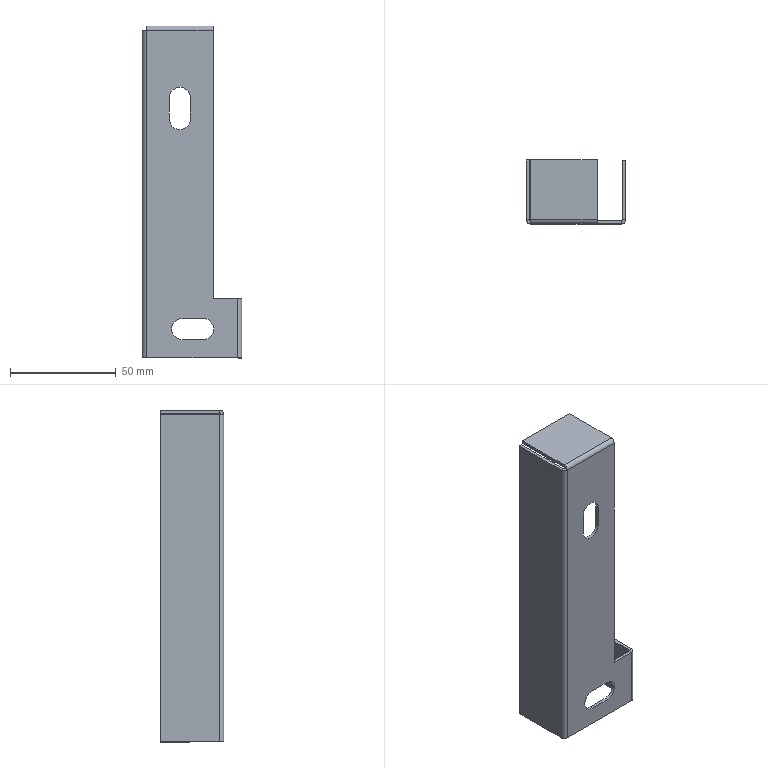Part | SolidWorks | features ICE 4, EdgeFlange 3, Cut 1, FlatPattern 1, SMBaseFlange 1, SheetMetal 1 | 1 solid | 41 faces | box 47 x 30 x 157 mm | volume 16912 mm3 | plane 30 | cylinder 11 | commonest cylinder face diameters 10 x5 1 x3 4 x3
STEP:
#1=CARTESIAN_POINT('',(17.75,0.,128.));
#2=VERTEX_POINT('',#1);
#3=CARTESIAN_POINT('',(22.75,0.,123.));
#4=VERTEX_POINT('',#3);
#5=CARTESIAN_POINT('',(17.75,0.,123.));
#6=DIRECTION('',(0.,1.,0.));
#7=DIRECTION('',(0.,0.,1.));
#8=AXIS2_PLACEMENT_3D('',#5,#6,#7);
#9=CIRCLE('',#8,5.);
#10=EDGE_CURVE('',#2,#4,#9,.T.);
#11=ORIENTED_EDGE('',*,*,#10,.F.);
#12=CARTESIAN_POINT('',(17.75,1.5,128.));
#13=VERTEX_POINT('',#12);
#14=CARTESIAN_POINT('',(17.75,-8.5,128.));
#15=DIRECTION('',(0.,1.,0.));
#16=VECTOR('',#15,1000.);
#17=LINE('',#14,#16);
#18=EDGE_CURVE('',#2,#13,#17,.T.);
#19=ORIENTED_EDGE('',*,*,#18,.T.);
#20=CARTESIAN_POINT('',(22.75,1.5,123.));
#21=VERTEX_POINT('',#20);
#22=CARTESIAN_POINT('',(17.75,1.5,123.));
#23=DIRECTION('',(0.,1.,0.));
#24=DIRECTION('',(0.,0.,1.));
#25=AXIS2_PLACEMENT_3D('',#22,#23,#24);
#26=CIRCLE('',#25,5.);
#27=EDGE_CURVE('',#13,#21,#26,.T.);
#28=ORIENTED_EDGE('',*,*,#27,.T.);
#29=CARTESIAN_POINT('',(22.75,-8.5,123.));
#30=DIRECTION('',(0.,1.,0.));
#31=VECTOR('',#30,1000.);
#32=LINE('',#29,#31);
#33=EDGE_CURVE('',#4,#21,#32,.T.);
#34=ORIENTED_EDGE('',*,*,#33,.F.);
#35=EDGE_LOOP('',(#11,#19,#28,#34));
#36=FACE_OUTER_BOUND('',#35,.T.);
#37=CARTESIAN_POINT('',(17.75,-8.5,123.));
#38=DIRECTION('',(0.,1.,0.));
#39=DIRECTION('',(0.,0.,1.));
#40=AXIS2_PLACEMENT_3D('',#37,#38,#39);
#41=CYLINDRICAL_SURFACE('',#40,5.);
#42=ADVANCED_FACE('',(#36),#41,.F.);
#43=CARTESIAN_POINT('',(33.5,1.5,28.));
#44=VERTEX_POINT('',#43);
#45=CARTESIAN_POINT('',(33.5,1.5,155.));
#46=VERTEX_POINT('',#45);
#47=CARTESIAN_POINT('',(33.5,1.5,155.));
#48=DIRECTION('',(0.,0.,1.));
#49=VECTOR('',#48,1000.);
#50=LINE('',#47,#49);
#51=EDGE_CURVE('',#44,#46,#50,.T.);
#52=ORIENTED_EDGE('',*,*,#51,.T.);
#53=CARTESIAN_POINT('',(33.5,0.,155.));
#54=VERTEX_POINT('',#53);
#55=CARTESIAN_POINT('',(33.5,1.5,155.));
#56=DIRECTION('',(0.,-1.,0.));
#57=VECTOR('',#56,1000.);
#58=LINE('',#55,#57);
#59=EDGE_CURVE('',#46,#54,#58,.T.);
#60=ORIENTED_EDGE('',*,*,#59,.T.);
#61=CARTESIAN_POINT('',(33.5,0.,28.));
#62=VERTEX_POINT('',#61);
#63=CARTESIAN_POINT('',(33.5,0.,157.));
#64=DIRECTION('',(0.,0.,1.));
#65=VECTOR('',#64,1000.);
#66=LINE('',#63,#65);
#67=EDGE_CURVE('',#62,#54,#66,.T.);
#68=ORIENTED_EDGE('',*,*,#67,.F.);
#69=CARTESIAN_POINT('',(33.5,0.,28.));
#70=DIRECTION('',(0.,1.,0.));
#71=VECTOR('',#70,1000.);
#72=LINE('',#69,#71);
#73=EDGE_CURVE('',#62,#44,#72,.T.);
#74=ORIENTED_EDGE('',*,*,#73,.T.);
#75=EDGE_LOOP('',(#52,#60,#68,#74));
#76=FACE_OUTER_BOUND('',#75,.T.);
#77=CARTESIAN_POINT('',(33.5,0.,157.));
#78=DIRECTION('',(-1.,0.,0.));
#79=DIRECTION('',(0.,0.,1.));
#80=AXIS2_PLACEMENT_3D('',#77,#78,#79);
#81=PLANE('',#80);
#82=ADVANCED_FACE('',(#76),#81,.F.);
#83=CARTESIAN_POINT('',(33.5,2.,157.));
#84=VERTEX_POINT('',#83);
#85=CARTESIAN_POINT('',(33.5,30.,157.));
#86=VERTEX_POINT('',#85);
#87=CARTESIAN_POINT('',(33.5,0.,157.));
#88=DIRECTION('',(0.,1.,0.));
#89=VECTOR('',#88,1000.);
#90=LINE('',#87,#89);
#91=EDGE_CURVE('',#84,#86,#90,.T.);
#92=ORIENTED_EDGE('',*,*,#91,.F.);
#93=CARTESIAN_POINT('',(33.5,2.,155.5));
#94=VERTEX_POINT('',#93);
#95=CARTESIAN_POINT('',(33.5,2.,157.));
#96=DIRECTION('',(0.,0.,-1.));
#97=VECTOR('',#96,1000.);
#98=LINE('',#95,#97);
#99=EDGE_CURVE('',#84,#94,#98,.T.);
#100=ORIENTED_EDGE('',*,*,#99,.T.);
#101=CARTESIAN_POINT('',(33.5,30.,155.5));
#102=VERTEX_POINT('',#101);
#103=CARTESIAN_POINT('',(33.5,0.,155.5));
#104=DIRECTION('',(0.,1.,0.));
#105=VECTOR('',#104,1000.);
#106=LINE('',#103,#105);
#107=EDGE_CURVE('',#94,#102,#106,.T.);
#108=ORIENTED_EDGE('',*,*,#107,.T.);
#109=CARTESIAN_POINT('',(33.5,30.,157.));
#110=DIRECTION('',(0.,0.,-1.));
#111=VECTOR('',#110,1000.);
#112=LINE('',#109,#111);
#113=EDGE_CURVE('',#86,#102,#112,.T.);
#114=ORIENTED_EDGE('',*,*,#113,.F.);
#115=EDGE_LOOP('',(#92,#100,#108,#114));
#116=FACE_OUTER_BOUND('',#115,.T.);
#117=CARTESIAN_POINT('',(33.5,0.,157.));
#118=DIRECTION('',(-1.,0.,0.));
#119=DIRECTION('',(0.,0.,1.));
#120=AXIS2_PLACEMENT_3D('',#117,#118,#119);
#121=PLANE('',#120);
#122=ADVANCED_FACE('',(#116),#121,.F.);
#123=CARTESIAN_POINT('',(0.,2.,155.));
#124=VERTEX_POINT('',#123);
#125=CARTESIAN_POINT('',(1.5,2.,155.));
#126=VERTEX_POINT('',#125);
#127=CARTESIAN_POINT('',(0.,2.,155.));
#128=DIRECTION('',(1.,0.,0.));
#129=VECTOR('',#128,1000.);
#130=LINE('',#127,#129);
#131=EDGE_CURVE('',#124,#126,#130,.T.);
#132=ORIENTED_EDGE('',*,*,#131,.F.);
#133=CARTESIAN_POINT('',(2.,0.,155.));
#134=VERTEX_POINT('',#133);
#135=CARTESIAN_POINT('',(2.,2.,155.));
#136=DIRECTION('',(0.,0.,1.));
#137=DIRECTION('',(-1.,0.,0.));
#138=AXIS2_PLACEMENT_3D('',#135,#136,#137);
#139=CIRCLE('',#138,2.);
#140=EDGE_CURVE('',#124,#134,#139,.T.);
#141=ORIENTED_EDGE('',*,*,#140,.T.);
#142=CARTESIAN_POINT('',(2.,1.5,155.));
#143=VERTEX_POINT('',#142);
#144=CARTESIAN_POINT('',(2.,1.5,155.));
#145=DIRECTION('',(0.,-1.,0.));
#146=VECTOR('',#145,1000.);
#147=LINE('',#144,#146);
#148=EDGE_CURVE('',#143,#134,#147,.T.);
#149=ORIENTED_EDGE('',*,*,#148,.F.);
#150=CARTESIAN_POINT('',(2.,2.,155.));
#151=DIRECTION('',(0.,0.,1.));
#152=DIRECTION('',(1.,0.,0.));
#153=AXIS2_PLACEMENT_3D('',#150,#151,#152);
#154=CIRCLE('',#153,0.5);
#155=EDGE_CURVE('',#126,#143,#154,.T.);
#156=ORIENTED_EDGE('',*,*,#155,.F.);
#157=EDGE_LOOP('',(#132,#141,#149,#156));
#158=FACE_OUTER_BOUND('',#157,.T.);
#159=CARTESIAN_POINT('',(0.,2.,155.));
#160=DIRECTION('',(0.,0.,1.));
#161=DIRECTION('',(1.,0.,0.));
#162=AXIS2_PLACEMENT_3D('',#159,#160,#161);
#163=PLANE('',#162);
#164=ADVANCED_FACE('',(#158),#163,.T.);
#165=CARTESIAN_POINT('',(0.,30.,155.));
#166=VERTEX_POINT('',#165);
#167=CARTESIAN_POINT('',(0.,30.,155.));
#168=DIRECTION('',(0.,-1.,0.));
#169=VECTOR('',#168,1000.);
#170=LINE('',#167,#169);
#171=EDGE_CURVE('',#166,#124,#170,.T.);
#172=ORIENTED_EDGE('',*,*,#171,.T.);
#173=ORIENTED_EDGE('',*,*,#131,.T.);
#174=CARTESIAN_POINT('',(1.5,30.,155.));
#175=VERTEX_POINT('',#174);
#176=CARTESIAN_POINT('',(1.5,30.,155.));
#177=DIRECTION('',(0.,-1.,0.));
#178=VECTOR('',#177,1000.);
#179=LINE('',#176,#178);
#180=EDGE_CURVE('',#175,#126,#179,.T.);
#181=ORIENTED_EDGE('',*,*,#180,.F.);
#182=CARTESIAN_POINT('',(0.,30.,155.));
#183=DIRECTION('',(1.,0.,0.));
#184=VECTOR('',#183,1000.);
#185=LINE('',#182,#184);
#186=EDGE_CURVE('',#166,#175,#185,.T.);
#187=ORIENTED_EDGE('',*,*,#186,.F.);
#188=EDGE_LOOP('',(#172,#173,#181,#187));
#189=FACE_OUTER_BOUND('',#188,.T.);
#190=CARTESIAN_POINT('',(2.,1.5,155.));
#191=DIRECTION('',(0.,0.,1.));
#192=DIRECTION('',(1.,0.,0.));
#193=AXIS2_PLACEMENT_3D('',#190,#191,#192);
#194=PLANE('',#193);
#195=ADVANCED_FACE('',(#189),#194,.T.);
#196=CARTESIAN_POINT('',(2.,0.,0.));
#197=VERTEX_POINT('',#196);
#198=CARTESIAN_POINT('',(2.,1.5,0.));
#199=VERTEX_POINT('',#198);
#200=CARTESIAN_POINT('',(2.,0.,0.));
#201=DIRECTION('',(0.,1.,0.));
#202=VECTOR('',#201,1000.);
#203=LINE('',#200,#202);
#204=EDGE_CURVE('',#197,#199,#203,.T.);
#205=ORIENTED_EDGE('',*,*,#204,.F.);
#206=CARTESIAN_POINT('',(0.,2.,0.));
#207=VERTEX_POINT('',#206);
#208=CARTESIAN_POINT('',(2.,2.,0.));
#209=DIRECTION('',(0.,0.,1.));
#210=DIRECTION('',(-1.,0.,0.));
#211=AXIS2_PLACEMENT_3D('',#208,#209,#210);
#212=CIRCLE('',#211,2.);
#213=EDGE_CURVE('',#207,#197,#212,.T.);
#214=ORIENTED_EDGE('',*,*,#213,.F.);
#215=CARTESIAN_POINT('',(1.5,2.,0.));
#216=VERTEX_POINT('',#215);
#217=CARTESIAN_POINT('',(1.5,2.,0.));
#218=DIRECTION('',(-1.,0.,0.));
#219=VECTOR('',#218,1000.);
#220=LINE('',#217,#219);
#221=EDGE_CURVE('',#216,#207,#220,.T.);
#222=ORIENTED_EDGE('',*,*,#221,.F.);
#223=CARTESIAN_POINT('',(2.,2.,0.));
#224=DIRECTION('',(0.,0.,1.));
#225=DIRECTION('',(1.,0.,0.));
#226=AXIS2_PLACEMENT_3D('',#223,#224,#225);
#227=CIRCLE('',#226,0.5);
#228=EDGE_CURVE('',#216,#199,#227,.T.);
#229=ORIENTED_EDGE('',*,*,#228,.T.);
#230=EDGE_LOOP('',(#205,#214,#222,#229));
#231=FACE_OUTER_BOUND('',#230,.T.);
#232=CARTESIAN_POINT('',(2.,0.,0.));
#233=DIRECTION('',(0.,0.,-1.));
#234=DIRECTION('',(-1.,0.,0.));
#235=AXIS2_PLACEMENT_3D('',#232,#233,#234);
#236=PLANE('',#235);
#237=ADVANCED_FACE('',(#231),#236,.T.);
#238=CARTESIAN_POINT('',(12.75,0.,113.));
#239=VERTEX_POINT('',#238);
#240=CARTESIAN_POINT('',(12.75,0.,123.));
#241=VERTEX_POINT('',#240);
#242=CARTESIAN_POINT('',(12.75,0.,155.));
#243=DIRECTION('',(0.,0.,1.));
#244=VECTOR('',#243,1000.);
#245=LINE('',#242,#244);
#246=EDGE_CURVE('',#239,#241,#245,.T.);
#247=ORIENTED_EDGE('',*,*,#246,.T.);
#248=CARTESIAN_POINT('',(17.75,0.,123.));
#249=DIRECTION('',(0.,1.,0.));
#250=DIRECTION('',(0.,0.,1.));
#251=AXIS2_PLACEMENT_3D('',#248,#249,#250);
#252=CIRCLE('',#251,5.);
#253=EDGE_CURVE('',#241,#2,#252,.T.);
#254=ORIENTED_EDGE('',*,*,#253,.T.);
#255=ORIENTED_EDGE('',*,*,#10,.T.);
#256=CARTESIAN_POINT('',(22.75,0.,113.));
#257=VERTEX_POINT('',#256);
#258=CARTESIAN_POINT('',(22.75,0.,155.));
#259=DIRECTION('',(0.,0.,-1.));
#260=VECTOR('',#259,1000.);
#261=LINE('',#258,#260);
#262=EDGE_CURVE('',#4,#257,#261,.T.);
#263=ORIENTED_EDGE('',*,*,#262,.T.);
#264=CARTESIAN_POINT('',(17.75,0.,113.));
#265=DIRECTION('',(0.,1.,0.));
#266=DIRECTION('',(0.,0.,1.));
#267=AXIS2_PLACEMENT_3D('',#264,#265,#266);
#268=CIRCLE('',#267,5.);
#269=EDGE_CURVE('',#257,#239,#268,.T.);
#270=ORIENTED_EDGE('',*,*,#269,.T.);
#271=EDGE_LOOP('',(#247,#254,#255,#263,#270));
#272=FACE_BOUND('',#271,.T.);
#273=CARTESIAN_POINT('',(28.8,0.,8.7));
#274=VERTEX_POINT('',#273);
#275=CARTESIAN_POINT('',(18.8,0.,8.7));
#276=VERTEX_POINT('',#275);
#277=CARTESIAN_POINT('',(0.,0.,8.7));
#278=DIRECTION('',(-1.,0.,0.));
#279=VECTOR('',#278,1000.);
#280=LINE('',#277,#279);
#281=EDGE_CURVE('',#274,#276,#280,.T.);
#282=ORIENTED_EDGE('',*,*,#281,.T.);
#283=CARTESIAN_POINT('',(18.8,0.,18.7));
#284=VERTEX_POINT('',#283);
#285=CARTESIAN_POINT('',(18.8,0.,13.7));
#286=DIRECTION('',(0.,1.,0.));
#287=DIRECTION('',(0.,0.,1.));
#288=AXIS2_PLACEMENT_3D('',#285,#286,#287);
#289=CIRCLE('',#288,5.);
#290=EDGE_CURVE('',#276,#284,#289,.T.);
#291=ORIENTED_EDGE('',*,*,#290,.T.);
#292=CARTESIAN_POINT('',(28.8,0.,18.7));
#293=VERTEX_POINT('',#292);
#294=CARTESIAN_POINT('',(0.,0.,18.7));
#295=DIRECTION('',(1.,0.,0.));
#296=VECTOR('',#295,1000.);
#297=LINE('',#294,#296);
#298=EDGE_CURVE('',#284,#293,#297,.T.);
#299=ORIENTED_EDGE('',*,*,#298,.T.);
#300=CARTESIAN_POINT('',(28.8,0.,13.7));
#301=DIRECTION('',(0.,1.,0.));
#302=DIRECTION('',(0.,0.,1.));
#303=AXIS2_PLACEMENT_3D('',#300,#301,#302);
#304=CIRCLE('',#303,5.);
#305=EDGE_CURVE('',#293,#274,#304,.T.);
#306=ORIENTED_EDGE('',*,*,#305,.T.);
#307=EDGE_LOOP('',(#282,#291,#299,#306));
#308=FACE_BOUND('',#307,.T.);
#309=CARTESIAN_POINT('',(45.,0.,28.));
#310=VERTEX_POINT('',#309);
#311=CARTESIAN_POINT('',(45.,0.,28.));
#312=DIRECTION('',(-1.,0.,0.));
#313=VECTOR('',#312,1000.);
#314=LINE('',#311,#313);
#315=EDGE_CURVE('',#310,#62,#314,.T.);
#316=ORIENTED_EDGE('',*,*,#315,.T.);
#317=ORIENTED_EDGE('',*,*,#67,.T.);
#318=CARTESIAN_POINT('',(0.,0.,155.));
#319=DIRECTION('',(1.,0.,0.));
#320=VECTOR('',#319,1000.);
#321=LINE('',#318,#320);
#322=EDGE_CURVE('',#134,#54,#321,.T.);
#323=ORIENTED_EDGE('',*,*,#322,.F.);
#324=CARTESIAN_POINT('',(2.,0.,155.));
#325=DIRECTION('',(0.,0.,-1.));
#326=VECTOR('',#325,1000.);
#327=LINE('',#324,#326);
#328=EDGE_CURVE('',#134,#197,#327,.T.);
#329=ORIENTED_EDGE('',*,*,#328,.T.);
#330=CARTESIAN_POINT('',(45.,0.,0.));
#331=VERTEX_POINT('',#330);
#332=CARTESIAN_POINT('',(0.,0.,0.));
#333=DIRECTION('',(1.,0.,0.));
#334=VECTOR('',#333,1000.);
#335=LINE('',#332,#334);
#336=EDGE_CURVE('',#197,#331,#335,.T.);
#337=ORIENTED_EDGE('',*,*,#336,.T.);
#338=CARTESIAN_POINT('',(45.,0.,155.));
#339=DIRECTION('',(0.,0.,-1.));
#340=VECTOR('',#339,1000.);
#341=LINE('',#338,#340);
#342=EDGE_CURVE('',#310,#331,#341,.T.);
#343=ORIENTED_EDGE('',*,*,#342,.F.);
#344=EDGE_LOOP('',(#316,#317,#323,#329,#337,#343));
#345=FACE_OUTER_BOUND('',#344,.T.);
#346=CARTESIAN_POINT('',(0.,0.,155.));
#347=DIRECTION('',(0.,1.,0.));
#348=DIRECTION('',(0.,0.,1.));
#349=AXIS2_PLACEMENT_3D('',#346,#347,#348);
#350=PLANE('',#349);
#351=ADVANCED_FACE('',(#272,#308,#345),#350,.F.);
#352=CARTESIAN_POINT('',(12.75,1.5,123.));
#353=VERTEX_POINT('',#352);
#354=CARTESIAN_POINT('',(17.75,1.5,123.));
#355=DIRECTION('',(0.,1.,0.));
#356=DIRECTION('',(0.,0.,1.));
#357=AXIS2_PLACEMENT_3D('',#354,#355,#356);
#358=CIRCLE('',#357,5.);
#359=EDGE_CURVE('',#353,#13,#358,.T.);
#360=ORIENTED_EDGE('',*,*,#359,.F.);
#361=CARTESIAN_POINT('',(12.75,1.5,113.));
#362=VERTEX_POINT('',#361);
#363=CARTESIAN_POINT('',(12.75,1.5,123.));
#364=DIRECTION('',(0.,0.,1.));
#365=VECTOR('',#364,1000.);
#366=LINE('',#363,#365);
#367=EDGE_CURVE('',#362,#353,#366,.T.);
#368=ORIENTED_EDGE('',*,*,#367,.F.);
#369=CARTESIAN_POINT('',(22.75,1.5,113.));
#370=VERTEX_POINT('',#369);
#371=CARTESIAN_POINT('',(17.75,1.5,113.));
#372=DIRECTION('',(0.,1.,0.));
#373=DIRECTION('',(0.,0.,1.));
#374=AXIS2_PLACEMENT_3D('',#371,#372,#373);
#375=CIRCLE('',#374,5.);
#376=EDGE_CURVE('',#370,#362,#375,.T.);
#377=ORIENTED_EDGE('',*,*,#376,.F.);
#378=CARTESIAN_POINT('',(22.75,1.5,123.));
#379=DIRECTION('',(0.,0.,-1.));
#380=VECTOR('',#379,1000.);
#381=LINE('',#378,#380);
#382=EDGE_CURVE('',#21,#370,#381,.T.);
#383=ORIENTED_EDGE('',*,*,#382,.F.);
#384=ORIENTED_EDGE('',*,*,#27,.F.);
#385=EDGE_LOOP('',(#360,#368,#377,#383,#384));
#386=FACE_BOUND('',#385,.T.);
#387=CARTESIAN_POINT('',(18.8,1.5,8.7));
#388=VERTEX_POINT('',#387);
#389=CARTESIAN_POINT('',(18.8,1.5,18.7));
#390=VERTEX_POINT('',#389);
#391=CARTESIAN_POINT('',(18.8,1.5,13.7));
#392=DIRECTION('',(0.,1.,0.));
#393=DIRECTION('',(0.,0.,1.));
#394=AXIS2_PLACEMENT_3D('',#391,#392,#393);
#395=CIRCLE('',#394,5.);
#396=EDGE_CURVE('',#388,#390,#395,.T.);
#397=ORIENTED_EDGE('',*,*,#396,.F.);
#398=CARTESIAN_POINT('',(28.8,1.5,8.7));
#399=VERTEX_POINT('',#398);
#400=CARTESIAN_POINT('',(18.8,1.5,8.7));
#401=DIRECTION('',(-1.,0.,0.));
#402=VECTOR('',#401,1000.);
#403=LINE('',#400,#402);
#404=EDGE_CURVE('',#399,#388,#403,.T.);
#405=ORIENTED_EDGE('',*,*,#404,.F.);
#406=CARTESIAN_POINT('',(28.8,1.5,18.7));
#407=VERTEX_POINT('',#406);
#408=CARTESIAN_POINT('',(28.8,1.5,13.7));
#409=DIRECTION('',(0.,1.,0.));
#410=DIRECTION('',(0.,0.,1.));
#411=AXIS2_PLACEMENT_3D('',#408,#409,#410);
#412=CIRCLE('',#411,5.);
#413=EDGE_CURVE('',#407,#399,#412,.T.);
#414=ORIENTED_EDGE('',*,*,#413,.F.);
#415=CARTESIAN_POINT('',(18.8,1.5,18.7));
#416=DIRECTION('',(1.,0.,0.));
#417=VECTOR('',#416,1000.);
#418=LINE('',#415,#417);
#419=EDGE_CURVE('',#390,#407,#418,.T.);
#420=ORIENTED_EDGE('',*,*,#419,.F.);
#421=EDGE_LOOP('',(#397,#405,#414,#420));
#422=FACE_BOUND('',#421,.T.);
#423=ORIENTED_EDGE('',*,*,#51,.F.);
#424=CARTESIAN_POINT('',(45.,1.5,28.));
#425=VERTEX_POINT('',#424);
#426=CARTESIAN_POINT('',(0.,1.5,28.));
#427=DIRECTION('',(-1.,0.,0.));
#428=VECTOR('',#427,1000.);
#429=LINE('',#426,#428);
#430=EDGE_CURVE('',#425,#44,#429,.T.);
#431=ORIENTED_EDGE('',*,*,#430,.F.);
#432=CARTESIAN_POINT('',(45.,1.5,0.));
#433=VERTEX_POINT('',#432);
#434=CARTESIAN_POINT('',(45.,1.5,155.));
#435=DIRECTION('',(0.,0.,-1.));
#436=VECTOR('',#435,1000.);
#437=LINE('',#434,#436);
#438=EDGE_CURVE('',#425,#433,#437,.T.);
#439=ORIENTED_EDGE('',*,*,#438,.T.);
#440=CARTESIAN_POINT('',(0.,1.5,0.));
#441=DIRECTION('',(1.,0.,0.));
#442=VECTOR('',#441,1000.);
#443=LINE('',#440,#442);
#444=EDGE_CURVE('',#199,#433,#443,.T.);
#445=ORIENTED_EDGE('',*,*,#444,.F.);
#446=CARTESIAN_POINT('',(2.,1.5,155.));
#447=DIRECTION('',(0.,0.,-1.));
#448=VECTOR('',#447,1000.);
#449=LINE('',#446,#448);
#450=EDGE_CURVE('',#143,#199,#449,.T.);
#451=ORIENTED_EDGE('',*,*,#450,.F.);
#452=CARTESIAN_POINT('',(0.,1.5,155.));
#453=DIRECTION('',(1.,0.,0.));
#454=VECTOR('',#453,1000.);
#455=LINE('',#452,#454);
#456=EDGE_CURVE('',#143,#46,#455,.T.);
#457=ORIENTED_EDGE('',*,*,#456,.T.);
#458=EDGE_LOOP('',(#423,#431,#439,#445,#451,#457));
#459=FACE_OUTER_BOUND('',#458,.T.);
#460=CARTESIAN_POINT('',(0.,1.5,155.));
#461=DIRECTION('',(0.,1.,0.));
#462=DIRECTION('',(0.,0.,1.));
#463=AXIS2_PLACEMENT_3D('',#460,#461,#462);
#464=PLANE('',#463);
#465=ADVANCED_FACE('',(#386,#422,#459),#464,.T.);
#466=ORIENTED_EDGE('',*,*,#228,.F.);
#467=CARTESIAN_POINT('',(1.5,2.,155.));
#468=DIRECTION('',(0.,0.,-1.));
#469=VECTOR('',#468,1000.);
#470=LINE('',#467,#469);
#471=EDGE_CURVE('',#126,#216,#470,.T.);
#472=ORIENTED_EDGE('',*,*,#471,.F.);
#473=ORIENTED_EDGE('',*,*,#155,.T.);
#474=ORIENTED_EDGE('',*,*,#450,.T.);
#475=EDGE_LOOP('',(#466,#472,#473,#474));
#476=FACE_OUTER_BOUND('',#475,.T.);
#477=CARTESIAN_POINT('',(2.,2.,155.));
#478=DIRECTION('',(0.,0.,-1.));
#479=DIRECTION('',(-1.,0.,0.));
#480=AXIS2_PLACEMENT_3D('',#477,#478,#479);
#481=CYLINDRICAL_SURFACE('',#480,0.5);
#482=ADVANCED_FACE('',(#476),#481,.F.);
#483=CARTESIAN_POINT('',(1.5,30.,0.));
#484=VERTEX_POINT('',#483);
#485=CARTESIAN_POINT('',(1.5,30.,0.));
#486=DIRECTION('',(0.,-1.,0.));
#487=VECTOR('',#486,1000.);
#488=LINE('',#485,#487);
#489=EDGE_CURVE('',#484,#216,#488,.T.);
#490=ORIENTED_EDGE('',*,*,#489,.F.);
#491=CARTESIAN_POINT('',(1.5,30.,155.));
#492=DIRECTION('',(0.,0.,-1.));
#493=VECTOR('',#492,1000.);
#494=LINE('',#491,#493);
#495=EDGE_CURVE('',#175,#484,#494,.T.);
#496=ORIENTED_EDGE('',*,*,#495,.F.);
#497=ORIENTED_EDGE('',*,*,#180,.T.);
#498=ORIENTED_EDGE('',*,*,#471,.T.);
#499=EDGE_LOOP('',(#490,#496,#497,#498));
#500=FACE_OUTER_BOUND('',#499,.T.);
#501=CARTESIAN_POINT('',(1.5,30.,155.));
#502=DIRECTION('',(1.,0.,0.));
#503=DIRECTION('',(0.,1.,0.));
#504=AXIS2_PLACEMENT_3D('',#501,#502,#503);
#505=PLANE('',#504);
#506=ADVANCED_FACE('',(#500),#505,.T.);
#507=CARTESIAN_POINT('',(0.,30.,0.));
#508=VERTEX_POINT('',#507);
#509=CARTESIAN_POINT('',(0.,30.,0.));
#510=DIRECTION('',(1.,0.,0.));
#511=VECTOR('',#510,1000.);
#512=LINE('',#509,#511);
#513=EDGE_CURVE('',#508,#484,#512,.T.);
#514=ORIENTED_EDGE('',*,*,#513,.F.);
#515=CARTESIAN_POINT('',(0.,30.,155.));
#516=DIRECTION('',(0.,0.,-1.));
#517=VECTOR('',#516,1000.);
#518=LINE('',#515,#517);
#519=EDGE_CURVE('',#166,#508,#518,.T.);
#520=ORIENTED_EDGE('',*,*,#519,.F.);
#521=ORIENTED_EDGE('',*,*,#186,.T.);
#522=ORIENTED_EDGE('',*,*,#495,.T.);
#523=EDGE_LOOP('',(#514,#520,#521,#522));
#524=FACE_OUTER_BOUND('',#523,.T.);
#525=CARTESIAN_POINT('',(0.,30.,155.));
#526=DIRECTION('',(0.,1.,0.));
#527=DIRECTION('',(0.,0.,1.));
#528=AXIS2_PLACEMENT_3D('',#525,#526,#527);
#529=PLANE('',#528);
#530=ADVANCED_FACE('',(#524),#529,.T.);
#531=CARTESIAN_POINT('',(0.,30.,0.));
#532=DIRECTION('',(0.,-1.,0.));
#533=VECTOR('',#532,1000.);
#534=LINE('',#531,#533);
#535=EDGE_CURVE('',#508,#207,#534,.T.);
#536=ORIENTED_EDGE('',*,*,#535,.T.);
#537=CARTESIAN_POINT('',(0.,2.,155.));
#538=DIRECTION('',(0.,0.,-1.));
#539=VECTOR('',#538,1000.);
#540=LINE('',#537,#539);
#541=EDGE_CURVE('',#124,#207,#540,.T.);
#542=ORIENTED_EDGE('',*,*,#541,.F.);
#543=ORIENTED_EDGE('',*,*,#171,.F.);
#544=ORIENTED_EDGE('',*,*,#519,.T.);
#545=EDGE_LOOP('',(#536,#542,#543,#544));
#546=FACE_OUTER_BOUND('',#545,.T.);
#547=CARTESIAN_POINT('',(0.,30.,155.));
#548=DIRECTION('',(1.,0.,0.));
#549=DIRECTION('',(0.,1.,0.));
#550=AXIS2_PLACEMENT_3D('',#547,#548,#549);
#551=PLANE('',#550);
#552=ADVANCED_FACE('',(#546),#551,.F.);
#553=ORIENTED_EDGE('',*,*,#213,.T.);
#554=ORIENTED_EDGE('',*,*,#328,.F.);
#555=ORIENTED_EDGE('',*,*,#140,.F.);
#556=ORIENTED_EDGE('',*,*,#541,.T.);
#557=EDGE_LOOP('',(#553,#554,#555,#556));
#558=FACE_OUTER_BOUND('',#557,.T.);
#559=CARTESIAN_POINT('',(2.,2.,155.));
#560=DIRECTION('',(0.,0.,-1.));
#561=DIRECTION('',(-1.,0.,0.));
#562=AXIS2_PLACEMENT_3D('',#559,#560,#561);
#563=CYLINDRICAL_SURFACE('',#562,2.);
#564=ADVANCED_FACE('',(#558),#563,.T.);
#565=ORIENTED_EDGE('',*,*,#489,.T.);
#566=ORIENTED_EDGE('',*,*,#221,.T.);
#567=ORIENTED_EDGE('',*,*,#535,.F.);
#568=ORIENTED_EDGE('',*,*,#513,.T.);
#569=EDGE_LOOP('',(#565,#566,#567,#568));
#570=FACE_OUTER_BOUND('',#569,.T.);
#571=CARTESIAN_POINT('',(2.,2.,0.));
#572=DIRECTION('',(0.,0.,1.));
#573=DIRECTION('',(1.,0.,0.));
#574=AXIS2_PLACEMENT_3D('',#571,#572,#573);
#575=PLANE('',#574);
#576=ADVANCED_FACE('',(#570),#575,.F.);
#577=CARTESIAN_POINT('',(2.,2.,155.5));
#578=VERTEX_POINT('',#577);
#579=CARTESIAN_POINT('',(2.,2.,157.));
#580=VERTEX_POINT('',#579);
#581=CARTESIAN_POINT('',(2.,2.,157.));
#582=DIRECTION('',(0.,0.,1.));
#583=VECTOR('',#582,1000.);
#584=LINE('',#581,#583);
#585=EDGE_CURVE('',#578,#580,#584,.T.);
#586=ORIENTED_EDGE('',*,*,#585,.F.);
#587=CARTESIAN_POINT('',(2.,2.,155.));
#588=DIRECTION('',(-1.,0.,0.));
#589=DIRECTION('',(0.,0.,-1.));
#590=AXIS2_PLACEMENT_3D('',#587,#588,#589);
#591=CIRCLE('',#590,0.5);
#592=EDGE_CURVE('',#143,#578,#591,.T.);
#593=ORIENTED_EDGE('',*,*,#592,.F.);
#594=ORIENTED_EDGE('',*,*,#148,.T.);
#595=CARTESIAN_POINT('',(2.,2.,155.));
#596=DIRECTION('',(-1.,0.,0.));
#597=DIRECTION('',(0.,0.,-1.));
#598=AXIS2_PLACEMENT_3D('',#595,#596,#597);
#599=CIRCLE('',#598,2.);
#600=EDGE_CURVE('',#134,#580,#599,.T.);
#601=ORIENTED_EDGE('',*,*,#600,.T.);
#602=EDGE_LOOP('',(#586,#593,#594,#601));
#603=FACE_OUTER_BOUND('',#602,.T.);
#604=CARTESIAN_POINT('',(2.,2.,155.));
#605=DIRECTION('',(-1.,0.,0.));
#606=DIRECTION('',(0.,0.,1.));
#607=AXIS2_PLACEMENT_3D('',#604,#605,#606);
#608=PLANE('',#607);
#609=ADVANCED_FACE('',(#603),#608,.T.);
#610=CARTESIAN_POINT('',(33.5,2.,155.));
#611=DIRECTION('',(1.,0.,0.));
#612=DIRECTION('',(0.,0.,1.));
#613=AXIS2_PLACEMENT_3D('',#610,#611,#612);
#614=CIRCLE('',#613,2.);
#615=EDGE_CURVE('',#84,#54,#614,.T.);
#616=ORIENTED_EDGE('',*,*,#615,.F.);
#617=CARTESIAN_POINT('',(2.,2.,157.));
#618=DIRECTION('',(-1.,0.,0.));
#619=VECTOR('',#618,1000.);
#620=LINE('',#617,#619);
#621=EDGE_CURVE('',#84,#580,#620,.T.);
#622=ORIENTED_EDGE('',*,*,#621,.T.);
#623=ORIENTED_EDGE('',*,*,#600,.F.);
#624=ORIENTED_EDGE('',*,*,#322,.T.);
#625=EDGE_LOOP('',(#616,#622,#623,#624));
#626=FACE_OUTER_BOUND('',#625,.T.);
#627=CARTESIAN_POINT('',(45.,2.,155.));
#628=DIRECTION('',(1.,0.,0.));
#629=DIRECTION('',(0.,0.,1.));
#630=AXIS2_PLACEMENT_3D('',#627,#628,#629);
#631=CYLINDRICAL_SURFACE('',#630,2.);
#632=ADVANCED_FACE('',(#626),#631,.T.);
#633=CARTESIAN_POINT('',(2.,2.,155.5));
#634=DIRECTION('',(1.,0.,0.));
#635=VECTOR('',#634,1000.);
#636=LINE('',#633,#635);
#637=EDGE_CURVE('',#578,#94,#636,.T.);
#638=ORIENTED_EDGE('',*,*,#637,.T.);
#639=CARTESIAN_POINT('',(33.5,2.,155.));
#640=DIRECTION('',(1.,0.,0.));
#641=DIRECTION('',(0.,0.,1.));
#642=AXIS2_PLACEMENT_3D('',#639,#640,#641);
#643=CIRCLE('',#642,0.5);
#644=EDGE_CURVE('',#94,#46,#643,.T.);
#645=ORIENTED_EDGE('',*,*,#644,.T.);
#646=ORIENTED_EDGE('',*,*,#456,.F.);
#647=ORIENTED_EDGE('',*,*,#592,.T.);
#648=EDGE_LOOP('',(#638,#645,#646,#647));
#649=FACE_OUTER_BOUND('',#648,.T.);
#650=CARTESIAN_POINT('',(45.,2.,155.));
#651=DIRECTION('',(1.,0.,0.));
#652=DIRECTION('',(0.,0.,1.));
#653=AXIS2_PLACEMENT_3D('',#650,#651,#652);
#654=CYLINDRICAL_SURFACE('',#653,0.5);
#655=ADVANCED_FACE('',(#649),#654,.F.);
#656=ORIENTED_EDGE('',*,*,#585,.T.);
#657=CARTESIAN_POINT('',(2.,30.,157.));
#658=VERTEX_POINT('',#657);
#659=CARTESIAN_POINT('',(2.,0.,157.));
#660=DIRECTION('',(0.,-1.,0.));
#661=VECTOR('',#660,1000.);
#662=LINE('',#659,#661);
#663=EDGE_CURVE('',#658,#580,#662,.T.);
#664=ORIENTED_EDGE('',*,*,#663,.F.);
#665=CARTESIAN_POINT('',(2.,30.,155.5));
#666=VERTEX_POINT('',#665);
#667=CARTESIAN_POINT('',(2.,30.,157.));
#668=DIRECTION('',(0.,0.,-1.));
#669=VECTOR('',#668,1000.);
#670=LINE('',#667,#669);
#671=EDGE_CURVE('',#658,#666,#670,.T.);
#672=ORIENTED_EDGE('',*,*,#671,.T.);
#673=CARTESIAN_POINT('',(2.,1.5,155.5));
#674=DIRECTION('',(0.,-1.,0.));
#675=VECTOR('',#674,1000.);
#676=LINE('',#673,#675);
#677=EDGE_CURVE('',#666,#578,#676,.T.);
#678=ORIENTED_EDGE('',*,*,#677,.T.);
#679=EDGE_LOOP('',(#656,#664,#672,#678));
#680=FACE_OUTER_BOUND('',#679,.T.);
#681=CARTESIAN_POINT('',(2.,1.5,157.));
#682=DIRECTION('',(1.,0.,0.));
#683=DIRECTION('',(0.,1.,0.));
#684=AXIS2_PLACEMENT_3D('',#681,#682,#683);
#685=PLANE('',#684);
#686=ADVANCED_FACE('',(#680),#685,.F.);
#687=ORIENTED_EDGE('',*,*,#621,.F.);
#688=ORIENTED_EDGE('',*,*,#91,.T.);
#689=CARTESIAN_POINT('',(0.,30.,157.));
#690=DIRECTION('',(-1.,0.,0.));
#691=VECTOR('',#690,1000.);
#692=LINE('',#689,#691);
#693=EDGE_CURVE('',#86,#658,#692,.T.);
#694=ORIENTED_EDGE('',*,*,#693,.T.);
#695=ORIENTED_EDGE('',*,*,#663,.T.);
#696=EDGE_LOOP('',(#687,#688,#694,#695));
#697=FACE_OUTER_BOUND('',#696,.T.);
#698=CARTESIAN_POINT('',(0.,0.,157.));
#699=DIRECTION('',(0.,0.,-1.));
#700=DIRECTION('',(-1.,0.,0.));
#701=AXIS2_PLACEMENT_3D('',#698,#699,#700);
#702=PLANE('',#701);
#703=ADVANCED_FACE('',(#697),#702,.F.);
#704=ORIENTED_EDGE('',*,*,#107,.F.);
#705=ORIENTED_EDGE('',*,*,#637,.F.);
#706=ORIENTED_EDGE('',*,*,#677,.F.);
#707=CARTESIAN_POINT('',(2.,30.,155.5));
#708=DIRECTION('',(-1.,0.,0.));
#709=VECTOR('',#708,1000.);
#710=LINE('',#707,#709);
#711=EDGE_CURVE('',#102,#666,#710,.T.);
#712=ORIENTED_EDGE('',*,*,#711,.F.);
#713=EDGE_LOOP('',(#704,#705,#706,#712));
#714=FACE_OUTER_BOUND('',#713,.T.);
#715=CARTESIAN_POINT('',(0.,0.,155.5));
#716=DIRECTION('',(0.,0.,-1.));
#717=DIRECTION('',(-1.,0.,0.));
#718=AXIS2_PLACEMENT_3D('',#715,#716,#717);
#719=PLANE('',#718);
#720=ADVANCED_FACE('',(#714),#719,.T.);
#721=ORIENTED_EDGE('',*,*,#693,.F.);
#722=ORIENTED_EDGE('',*,*,#113,.T.);
#723=ORIENTED_EDGE('',*,*,#711,.T.);
#724=ORIENTED_EDGE('',*,*,#671,.F.);
#725=EDGE_LOOP('',(#721,#722,#723,#724));
#726=FACE_OUTER_BOUND('',#725,.T.);
#727=CARTESIAN_POINT('',(2.,30.,157.));
#728=DIRECTION('',(0.,-1.,0.));
#729=DIRECTION('',(0.,0.,-1.));
#730=AXIS2_PLACEMENT_3D('',#727,#728,#729);
#731=PLANE('',#730);
#732=ADVANCED_FACE('',(#726),#731,.F.);
#733=ORIENTED_EDGE('',*,*,#59,.F.);
#734=ORIENTED_EDGE('',*,*,#644,.F.);
#735=ORIENTED_EDGE('',*,*,#99,.F.);
#736=ORIENTED_EDGE('',*,*,#615,.T.);
#737=EDGE_LOOP('',(#733,#734,#735,#736));
#738=FACE_OUTER_BOUND('',#737,.T.);
#739=CARTESIAN_POINT('',(33.5,0.,157.));
#740=DIRECTION('',(-1.,0.,0.));
#741=DIRECTION('',(0.,0.,1.));
#742=AXIS2_PLACEMENT_3D('',#739,#740,#741);
#743=PLANE('',#742);
#744=ADVANCED_FACE('',(#738),#743,.F.);
#745=ORIENTED_EDGE('',*,*,#430,.T.);
#746=ORIENTED_EDGE('',*,*,#73,.F.);
#747=ORIENTED_EDGE('',*,*,#315,.F.);
#748=CARTESIAN_POINT('',(45.,0.,28.));
#749=DIRECTION('',(0.,1.,0.));
#750=VECTOR('',#749,1000.);
#751=LINE('',#748,#750);
#752=EDGE_CURVE('',#310,#425,#751,.T.);
#753=ORIENTED_EDGE('',*,*,#752,.T.);
#754=EDGE_LOOP('',(#745,#746,#747,#753));
#755=FACE_OUTER_BOUND('',#754,.T.);
#756=CARTESIAN_POINT('',(45.,0.,28.));
#757=DIRECTION('',(0.,0.,-1.));
#758=DIRECTION('',(-1.,0.,0.));
#759=AXIS2_PLACEMENT_3D('',#756,#757,#758);
#760=PLANE('',#759);
#761=ADVANCED_FACE('',(#755),#760,.F.);
#762=CARTESIAN_POINT('',(18.8,-8.5,8.7));
#763=DIRECTION('',(0.,1.,0.));
#764=VECTOR('',#763,1000.);
#765=LINE('',#762,#764);
#766=EDGE_CURVE('',#276,#388,#765,.T.);
#767=ORIENTED_EDGE('',*,*,#766,.T.);
#768=ORIENTED_EDGE('',*,*,#396,.T.);
#769=CARTESIAN_POINT('',(18.8,-8.5,18.7));
#770=DIRECTION('',(0.,1.,0.));
#771=VECTOR('',#770,1000.);
#772=LINE('',#769,#771);
#773=EDGE_CURVE('',#284,#390,#772,.T.);
#774=ORIENTED_EDGE('',*,*,#773,.F.);
#775=ORIENTED_EDGE('',*,*,#290,.F.);
#776=EDGE_LOOP('',(#767,#768,#774,#775));
#777=FACE_OUTER_BOUND('',#776,.T.);
#778=CARTESIAN_POINT('',(18.8,-8.5,13.7));
#779=DIRECTION('',(0.,1.,0.));
#780=DIRECTION('',(0.,0.,1.));
#781=AXIS2_PLACEMENT_3D('',#778,#779,#780);
#782=CYLINDRICAL_SURFACE('',#781,5.);
#783=ADVANCED_FACE('',(#777),#782,.F.);
#784=CARTESIAN_POINT('',(28.8,-8.5,8.7));
#785=DIRECTION('',(0.,1.,0.));
#786=VECTOR('',#785,1000.);
#787=LINE('',#784,#786);
#788=EDGE_CURVE('',#274,#399,#787,.T.);
#789=ORIENTED_EDGE('',*,*,#788,.T.);
#790=ORIENTED_EDGE('',*,*,#404,.T.);
#791=ORIENTED_EDGE('',*,*,#766,.F.);
#792=ORIENTED_EDGE('',*,*,#281,.F.);
#793=EDGE_LOOP('',(#789,#790,#791,#792));
#794=FACE_OUTER_BOUND('',#793,.T.);
#795=CARTESIAN_POINT('',(18.8,-8.5,8.7));
#796=DIRECTION('',(0.,0.,-1.));
#797=DIRECTION('',(-1.,0.,0.));
#798=AXIS2_PLACEMENT_3D('',#795,#796,#797);
#799=PLANE('',#798);
#800=ADVANCED_FACE('',(#794),#799,.F.);
#801=CARTESIAN_POINT('',(28.8,-8.5,18.7));
#802=DIRECTION('',(0.,1.,0.));
#803=VECTOR('',#802,1000.);
#804=LINE('',#801,#803);
#805=EDGE_CURVE('',#293,#407,#804,.T.);
#806=ORIENTED_EDGE('',*,*,#805,.T.);
#807=ORIENTED_EDGE('',*,*,#413,.T.);
#808=ORIENTED_EDGE('',*,*,#788,.F.);
#809=ORIENTED_EDGE('',*,*,#305,.F.);
#810=EDGE_LOOP('',(#806,#807,#808,#809));
#811=FACE_OUTER_BOUND('',#810,.T.);
#812=CARTESIAN_POINT('',(28.8,-8.5,13.7));
#813=DIRECTION('',(0.,1.,0.));
#814=DIRECTION('',(0.,0.,1.));
#815=AXIS2_PLACEMENT_3D('',#812,#813,#814);
#816=CYLINDRICAL_SURFACE('',#815,5.);
#817=ADVANCED_FACE('',(#811),#816,.F.);
#818=ORIENTED_EDGE('',*,*,#773,.T.);
#819=ORIENTED_EDGE('',*,*,#419,.T.);
#820=ORIENTED_EDGE('',*,*,#805,.F.);
#821=ORIENTED_EDGE('',*,*,#298,.F.);
#822=EDGE_LOOP('',(#818,#819,#820,#821));
#823=FACE_OUTER_BOUND('',#822,.T.);
#824=CARTESIAN_POINT('',(18.8,-8.5,18.7));
#825=DIRECTION('',(0.,0.,1.));
#826=DIRECTION('',(1.,0.,0.));
#827=AXIS2_PLACEMENT_3D('',#824,#825,#826);
#828=PLANE('',#827);
#829=ADVANCED_FACE('',(#823),#828,.F.);
#830=ORIENTED_EDGE('',*,*,#18,.F.);
#831=ORIENTED_EDGE('',*,*,#253,.F.);
#832=CARTESIAN_POINT('',(12.75,-8.5,123.));
#833=DIRECTION('',(0.,1.,0.));
#834=VECTOR('',#833,1000.);
#835=LINE('',#832,#834);
#836=EDGE_CURVE('',#241,#353,#835,.T.);
#837=ORIENTED_EDGE('',*,*,#836,.T.);
#838=ORIENTED_EDGE('',*,*,#359,.T.);
#839=EDGE_LOOP('',(#830,#831,#837,#838));
#840=FACE_OUTER_BOUND('',#839,.T.);
#841=CARTESIAN_POINT('',(17.75,-8.5,123.));
#842=DIRECTION('',(0.,1.,0.));
#843=DIRECTION('',(0.,0.,1.));
#844=AXIS2_PLACEMENT_3D('',#841,#842,#843);
#845=CYLINDRICAL_SURFACE('',#844,5.);
#846=ADVANCED_FACE('',(#840),#845,.F.);
#847=CARTESIAN_POINT('',(12.75,-8.5,113.));
#848=DIRECTION('',(0.,1.,0.));
#849=VECTOR('',#848,1000.);
#850=LINE('',#847,#849);
#851=EDGE_CURVE('',#239,#362,#850,.T.);
#852=ORIENTED_EDGE('',*,*,#851,.T.);
#853=ORIENTED_EDGE('',*,*,#367,.T.);
#854=ORIENTED_EDGE('',*,*,#836,.F.);
#855=ORIENTED_EDGE('',*,*,#246,.F.);
#856=EDGE_LOOP('',(#852,#853,#854,#855));
#857=FACE_OUTER_BOUND('',#856,.T.);
#858=CARTESIAN_POINT('',(12.75,-8.5,123.));
#859=DIRECTION('',(-1.,0.,0.));
#860=DIRECTION('',(0.,0.,1.));
#861=AXIS2_PLACEMENT_3D('',#858,#859,#860);
#862=PLANE('',#861);
#863=ADVANCED_FACE('',(#857),#862,.F.);
#864=CARTESIAN_POINT('',(22.75,-8.5,113.));
#865=DIRECTION('',(0.,1.,0.));
#866=VECTOR('',#865,1000.);
#867=LINE('',#864,#866);
#868=EDGE_CURVE('',#257,#370,#867,.T.);
#869=ORIENTED_EDGE('',*,*,#868,.T.);
#870=ORIENTED_EDGE('',*,*,#376,.T.);
#871=ORIENTED_EDGE('',*,*,#851,.F.);
#872=ORIENTED_EDGE('',*,*,#269,.F.);
#873=EDGE_LOOP('',(#869,#870,#871,#872));
#874=FACE_OUTER_BOUND('',#873,.T.);
#875=CARTESIAN_POINT('',(17.75,-8.5,113.));
#876=DIRECTION('',(0.,1.,0.));
#877=DIRECTION('',(0.,0.,1.));
#878=AXIS2_PLACEMENT_3D('',#875,#876,#877);
#879=CYLINDRICAL_SURFACE('',#878,5.);
#880=ADVANCED_FACE('',(#874),#879,.F.);
#881=ORIENTED_EDGE('',*,*,#33,.T.);
#882=ORIENTED_EDGE('',*,*,#382,.T.);
#883=ORIENTED_EDGE('',*,*,#868,.F.);
#884=ORIENTED_EDGE('',*,*,#262,.F.);
#885=EDGE_LOOP('',(#881,#882,#883,#884));
#886=FACE_OUTER_BOUND('',#885,.T.);
#887=CARTESIAN_POINT('',(22.75,-8.5,123.));
#888=DIRECTION('',(1.,0.,0.));
#889=DIRECTION('',(0.,0.,-1.));
#890=AXIS2_PLACEMENT_3D('',#887,#888,#889);
#891=PLANE('',#890);
#892=ADVANCED_FACE('',(#886),#891,.F.);
#893=CARTESIAN_POINT('',(45.5,2.,28.));
#894=VERTEX_POINT('',#893);
#895=CARTESIAN_POINT('',(47.,2.,28.));
#896=VERTEX_POINT('',#895);
#897=CARTESIAN_POINT('',(47.,2.,28.));
#898=DIRECTION('',(1.,0.,0.));
#899=VECTOR('',#898,1000.);
#900=LINE('',#897,#899);
#901=EDGE_CURVE('',#894,#896,#900,.T.);
#902=ORIENTED_EDGE('',*,*,#901,.F.);
#903=CARTESIAN_POINT('',(45.,2.,28.));
#904=DIRECTION('',(0.,0.,1.));
#905=DIRECTION('',(-1.,0.,0.));
#906=AXIS2_PLACEMENT_3D('',#903,#904,#905);
#907=CIRCLE('',#906,0.5);
#908=EDGE_CURVE('',#425,#894,#907,.T.);
#909=ORIENTED_EDGE('',*,*,#908,.F.);
#910=ORIENTED_EDGE('',*,*,#752,.F.);
#911=CARTESIAN_POINT('',(45.,2.,28.));
#912=DIRECTION('',(0.,0.,1.));
#913=DIRECTION('',(-1.,0.,0.));
#914=AXIS2_PLACEMENT_3D('',#911,#912,#913);
#915=CIRCLE('',#914,2.);
#916=EDGE_CURVE('',#310,#896,#915,.T.);
#917=ORIENTED_EDGE('',*,*,#916,.T.);
#918=EDGE_LOOP('',(#902,#909,#910,#917));
#919=FACE_OUTER_BOUND('',#918,.T.);
#920=CARTESIAN_POINT('',(45.,2.,28.));
#921=DIRECTION('',(0.,0.,1.));
#922=DIRECTION('',(1.,0.,0.));
#923=AXIS2_PLACEMENT_3D('',#920,#921,#922);
#924=PLANE('',#923);
#925=ADVANCED_FACE('',(#919),#924,.T.);
#926=CARTESIAN_POINT('',(45.5,2.,0.));
#927=VERTEX_POINT('',#926);
#928=CARTESIAN_POINT('',(45.,2.,0.));
#929=DIRECTION('',(0.,0.,-1.));
#930=DIRECTION('',(-1.,0.,0.));
#931=AXIS2_PLACEMENT_3D('',#928,#929,#930);
#932=CIRCLE('',#931,0.5);
#933=EDGE_CURVE('',#927,#433,#932,.T.);
#934=ORIENTED_EDGE('',*,*,#933,.F.);
#935=CARTESIAN_POINT('',(47.,2.,0.));
#936=VERTEX_POINT('',#935);
#937=CARTESIAN_POINT('',(45.5,2.,0.));
#938=DIRECTION('',(1.,0.,0.));
#939=VECTOR('',#938,1000.);
#940=LINE('',#937,#939);
#941=EDGE_CURVE('',#927,#936,#940,.T.);
#942=ORIENTED_EDGE('',*,*,#941,.T.);
#943=CARTESIAN_POINT('',(45.,2.,0.));
#944=DIRECTION('',(0.,0.,-1.));
#945=DIRECTION('',(-1.,0.,0.));
#946=AXIS2_PLACEMENT_3D('',#943,#944,#945);
#947=CIRCLE('',#946,2.);
#948=EDGE_CURVE('',#936,#331,#947,.T.);
#949=ORIENTED_EDGE('',*,*,#948,.T.);
#950=CARTESIAN_POINT('',(45.,1.5,0.));
#951=DIRECTION('',(0.,-1.,0.));
#952=VECTOR('',#951,1000.);
#953=LINE('',#950,#952);
#954=EDGE_CURVE('',#433,#331,#953,.T.);
#955=ORIENTED_EDGE('',*,*,#954,.F.);
#956=EDGE_LOOP('',(#934,#942,#949,#955));
#957=FACE_OUTER_BOUND('',#956,.T.);
#958=CARTESIAN_POINT('',(45.,2.,0.));
#959=DIRECTION('',(0.,0.,1.));
#960=DIRECTION('',(1.,0.,0.));
#961=AXIS2_PLACEMENT_3D('',#958,#959,#960);
#962=PLANE('',#961);
#963=ADVANCED_FACE('',(#957),#962,.F.);
#964=ORIENTED_EDGE('',*,*,#342,.T.);
#965=ORIENTED_EDGE('',*,*,#948,.F.);
#966=CARTESIAN_POINT('',(47.,2.,28.));
#967=DIRECTION('',(0.,0.,1.));
#968=VECTOR('',#967,1000.);
#969=LINE('',#966,#968);
#970=EDGE_CURVE('',#936,#896,#969,.T.);
#971=ORIENTED_EDGE('',*,*,#970,.T.);
#972=ORIENTED_EDGE('',*,*,#916,.F.);
#973=EDGE_LOOP('',(#964,#965,#971,#972));
#974=FACE_OUTER_BOUND('',#973,.T.);
#975=CARTESIAN_POINT('',(45.,2.,0.));
#976=DIRECTION('',(0.,0.,-1.));
#977=DIRECTION('',(1.,0.,0.));
#978=AXIS2_PLACEMENT_3D('',#975,#976,#977);
#979=CYLINDRICAL_SURFACE('',#978,2.);
#980=ADVANCED_FACE('',(#974),#979,.T.);
#981=ORIENTED_EDGE('',*,*,#438,.F.);
#982=ORIENTED_EDGE('',*,*,#908,.T.);
#983=CARTESIAN_POINT('',(45.5,2.,28.));
#984=DIRECTION('',(0.,0.,-1.));
#985=VECTOR('',#984,1000.);
#986=LINE('',#983,#985);
#987=EDGE_CURVE('',#894,#927,#986,.T.);
#988=ORIENTED_EDGE('',*,*,#987,.T.);
#989=ORIENTED_EDGE('',*,*,#933,.T.);
#990=EDGE_LOOP('',(#981,#982,#988,#989));
#991=FACE_OUTER_BOUND('',#990,.T.);
#992=CARTESIAN_POINT('',(45.,2.,0.));
#993=DIRECTION('',(0.,0.,-1.));
#994=DIRECTION('',(1.,0.,0.));
#995=AXIS2_PLACEMENT_3D('',#992,#993,#994);
#996=CYLINDRICAL_SURFACE('',#995,0.5);
#997=ADVANCED_FACE('',(#991),#996,.F.);
#998=ORIENTED_EDGE('',*,*,#901,.T.);
#999=CARTESIAN_POINT('',(47.,30.,28.));
#1000=VERTEX_POINT('',#999);
#1001=CARTESIAN_POINT('',(47.,0.,28.));
#1002=DIRECTION('',(0.,-1.,0.));
#1003=VECTOR('',#1002,1000.);
#1004=LINE('',#1001,#1003);
#1005=EDGE_CURVE('',#1000,#896,#1004,.T.);
#1006=ORIENTED_EDGE('',*,*,#1005,.F.);
#1007=CARTESIAN_POINT('',(45.5,30.,28.));
#1008=VERTEX_POINT('',#1007);
#1009=CARTESIAN_POINT('',(47.,30.,28.));
#1010=DIRECTION('',(-1.,0.,0.));
#1011=VECTOR('',#1010,1000.);
#1012=LINE('',#1009,#1011);
#1013=EDGE_CURVE('',#1000,#1008,#1012,.T.);
#1014=ORIENTED_EDGE('',*,*,#1013,.T.);
#1015=CARTESIAN_POINT('',(45.5,1.5,28.));
#1016=DIRECTION('',(0.,-1.,0.));
#1017=VECTOR('',#1016,1000.);
#1018=LINE('',#1015,#1017);
#1019=EDGE_CURVE('',#1008,#894,#1018,.T.);
#1020=ORIENTED_EDGE('',*,*,#1019,.T.);
#1021=EDGE_LOOP('',(#998,#1006,#1014,#1020));
#1022=FACE_OUTER_BOUND('',#1021,.T.);
#1023=CARTESIAN_POINT('',(47.,1.5,28.));
#1024=DIRECTION('',(0.,0.,-1.));
#1025=DIRECTION('',(0.,1.,0.));
#1026=AXIS2_PLACEMENT_3D('',#1023,#1024,#1025);
#1027=PLANE('',#1026);
#1028=ADVANCED_FACE('',(#1022),#1027,.F.);
#1029=ORIENTED_EDGE('',*,*,#941,.F.);
#1030=CARTESIAN_POINT('',(45.5,30.,0.));
#1031=VERTEX_POINT('',#1030);
#1032=CARTESIAN_POINT('',(45.5,30.,0.));
#1033=DIRECTION('',(0.,1.,0.));
#1034=VECTOR('',#1033,1000.);
#1035=LINE('',#1032,#1034);
#1036=EDGE_CURVE('',#927,#1031,#1035,.T.);
#1037=ORIENTED_EDGE('',*,*,#1036,.T.);
#1038=CARTESIAN_POINT('',(47.,30.,0.));
#1039=VERTEX_POINT('',#1038);
#1040=CARTESIAN_POINT('',(47.,30.,0.));
#1041=DIRECTION('',(-1.,0.,0.));
#1042=VECTOR('',#1041,1000.);
#1043=LINE('',#1040,#1042);
#1044=EDGE_CURVE('',#1039,#1031,#1043,.T.);
#1045=ORIENTED_EDGE('',*,*,#1044,.F.);
#1046=CARTESIAN_POINT('',(47.,0.,0.));
#1047=DIRECTION('',(0.,1.,0.));
#1048=VECTOR('',#1047,1000.);
#1049=LINE('',#1046,#1048);
#1050=EDGE_CURVE('',#936,#1039,#1049,.T.);
#1051=ORIENTED_EDGE('',*,*,#1050,.F.);
#1052=EDGE_LOOP('',(#1029,#1037,#1045,#1051));
#1053=FACE_OUTER_BOUND('',#1052,.T.);
#1054=CARTESIAN_POINT('',(47.,30.,0.));
#1055=DIRECTION('',(0.,0.,1.));
#1056=DIRECTION('',(0.,-1.,0.));
#1057=AXIS2_PLACEMENT_3D('',#1054,#1055,#1056);
#1058=PLANE('',#1057);
#1059=ADVANCED_FACE('',(#1053),#1058,.F.);
#1060=ORIENTED_EDGE('',*,*,#970,.F.);
#1061=ORIENTED_EDGE('',*,*,#1050,.T.);
#1062=CARTESIAN_POINT('',(47.,30.,0.));
#1063=DIRECTION('',(0.,0.,1.));
#1064=VECTOR('',#1063,1000.);
#1065=LINE('',#1062,#1064);
#1066=EDGE_CURVE('',#1039,#1000,#1065,.T.);
#1067=ORIENTED_EDGE('',*,*,#1066,.T.);
#1068=ORIENTED_EDGE('',*,*,#1005,.T.);
#1069=EDGE_LOOP('',(#1060,#1061,#1067,#1068));
#1070=FACE_OUTER_BOUND('',#1069,.T.);
#1071=CARTESIAN_POINT('',(47.,0.,0.));
#1072=DIRECTION('',(-1.,0.,0.));
#1073=DIRECTION('',(0.,-1.,0.));
#1074=AXIS2_PLACEMENT_3D('',#1071,#1072,#1073);
#1075=PLANE('',#1074);
#1076=ADVANCED_FACE('',(#1070),#1075,.F.);
#1077=ORIENTED_EDGE('',*,*,#1036,.F.);
#1078=ORIENTED_EDGE('',*,*,#987,.F.);
#1079=ORIENTED_EDGE('',*,*,#1019,.F.);
#1080=CARTESIAN_POINT('',(45.5,30.,28.));
#1081=DIRECTION('',(0.,0.,1.));
#1082=VECTOR('',#1081,1000.);
#1083=LINE('',#1080,#1082);
#1084=EDGE_CURVE('',#1031,#1008,#1083,.T.);
#1085=ORIENTED_EDGE('',*,*,#1084,.F.);
#1086=EDGE_LOOP('',(#1077,#1078,#1079,#1085));
#1087=FACE_OUTER_BOUND('',#1086,.T.);
#1088=CARTESIAN_POINT('',(45.5,0.,0.));
#1089=DIRECTION('',(-1.,0.,0.));
#1090=DIRECTION('',(0.,-1.,0.));
#1091=AXIS2_PLACEMENT_3D('',#1088,#1089,#1090);
#1092=PLANE('',#1091);
#1093=ADVANCED_FACE('',(#1087),#1092,.T.);
#1094=ORIENTED_EDGE('',*,*,#1084,.T.);
#1095=ORIENTED_EDGE('',*,*,#1013,.F.);
#1096=ORIENTED_EDGE('',*,*,#1066,.F.);
#1097=ORIENTED_EDGE('',*,*,#1044,.T.);
#1098=EDGE_LOOP('',(#1094,#1095,#1096,#1097));
#1099=FACE_OUTER_BOUND('',#1098,.T.);
#1100=CARTESIAN_POINT('',(47.,30.,28.));
#1101=DIRECTION('',(0.,-1.,0.));
#1102=DIRECTION('',(1.,0.,0.));
#1103=AXIS2_PLACEMENT_3D('',#1100,#1101,#1102);
#1104=PLANE('',#1103);
#1105=ADVANCED_FACE('',(#1099),#1104,.F.);
#1106=ORIENTED_EDGE('',*,*,#954,.T.);
#1107=ORIENTED_EDGE('',*,*,#336,.F.);
#1108=ORIENTED_EDGE('',*,*,#204,.T.);
#1109=ORIENTED_EDGE('',*,*,#444,.T.);
#1110=EDGE_LOOP('',(#1106,#1107,#1108,#1109));
#1111=FACE_OUTER_BOUND('',#1110,.T.);
#1112=CARTESIAN_POINT('',(2.,0.,0.));
#1113=DIRECTION('',(0.,0.,1.));
#1114=DIRECTION('',(1.,0.,0.));
#1115=AXIS2_PLACEMENT_3D('',#1112,#1113,#1114);
#1116=PLANE('',#1115);
#1117=ADVANCED_FACE('',(#1111),#1116,.F.);
#1118=CLOSED_SHELL('',(#42,#82,#122,#164,#195,#237,#351,#465,#482,#506,#530,#552,#564,#576,#609,#632,#655,#686,#703,#720,#732,#744,#761,#783,#800,#817,#829,#846,#863,#880,#892,#925,#963,#980,#997,#1028,#1059,#1076,#1093,#1105,#1117));
#1119=MANIFOLD_SOLID_BREP('',#1118);
#1120=CARTESIAN_POINT('',(0.,0.,0.));
#1121=DIRECTION('',(0.,0.,1.));
#1122=DIRECTION('',(1.,0.,0.));
#1123=AXIS2_PLACEMENT_3D('',#1120,#1121,#1122);
#1124=(LENGTH_UNIT()NAMED_UNIT(*)SI_UNIT(.MILLI.,.METRE.));
#1125=UNCERTAINTY_MEASURE_WITH_UNIT(LENGTH_MEASURE(0.00001),#1124,'','');
#1126=(NAMED_UNIT(*)PLANE_ANGLE_UNIT()SI_UNIT($,.RADIAN.));
#1127=(NAMED_UNIT(*)SI_UNIT($,.STERADIAN.)SOLID_ANGLE_UNIT());
#1128=(GEOMETRIC_REPRESENTATION_CONTEXT(3)GLOBAL_UNCERTAINTY_ASSIGNED_CONTEXT((#1125))GLOBAL_UNIT_ASSIGNED_CONTEXT((#1124,#1126,#1127))REPRESENTATION_CONTEXT('',''));
#1129=ADVANCED_BREP_SHAPE_REPRESENTATION('',(#1119,#1123),#1128);